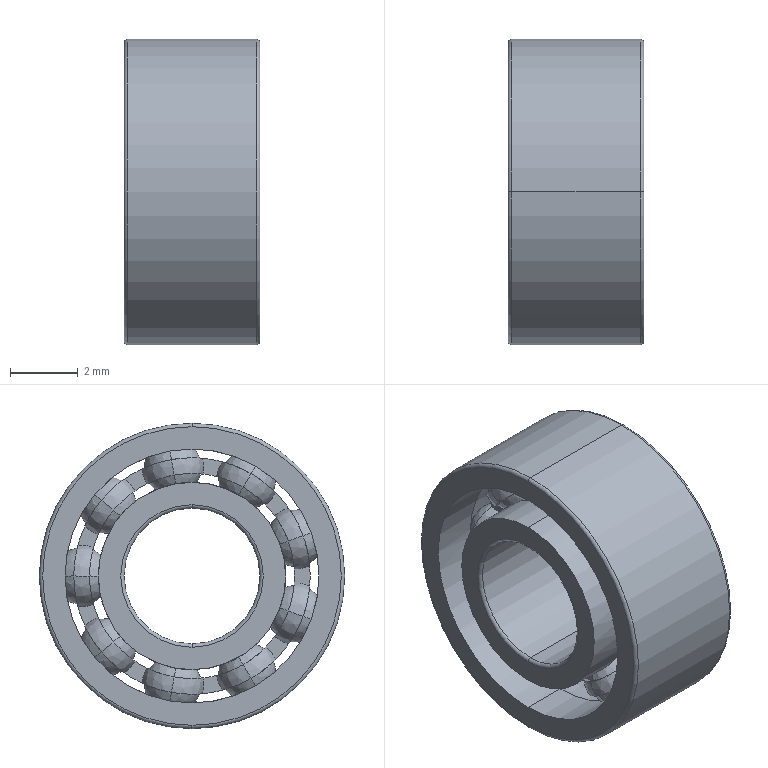Part | SolidWorks | features Revolution 5, CirPattern 2, RevCut 2 | 1 solid | 148 faces | box 4 x 9 x 9 mm | volume 135.884 mm3 | sphere 72 | torus 38 | plane 22 | cylinder 16 | commonest cylinder face diameters 5.52 x4 7.48 x4 4 x2 6.038 x2 6.962 x2 9 x2